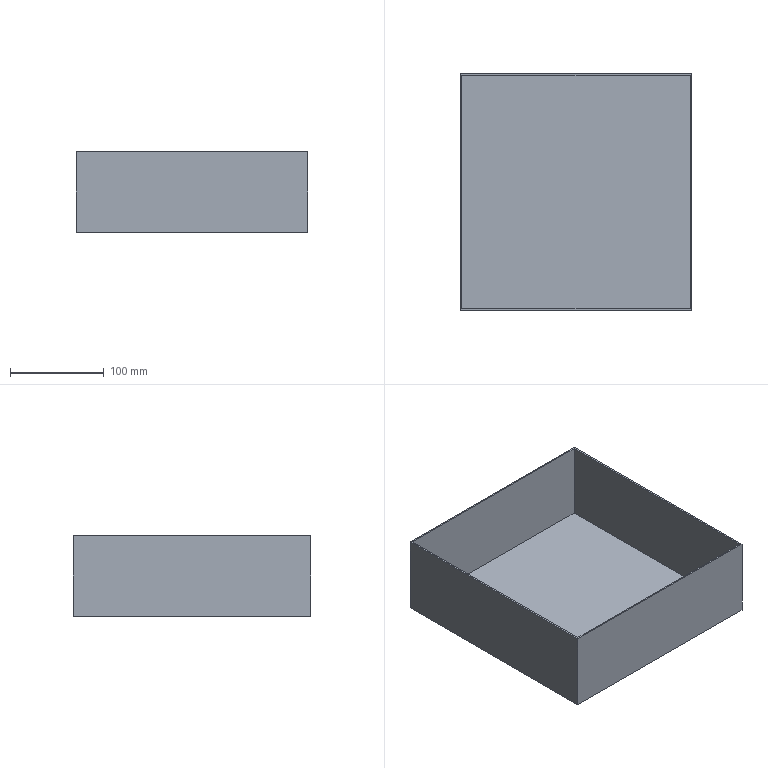Part | STEP file | 012-6-07-011 | 1 solid | 11 faces | box 247 x 253 x 86 mm | volume 291638 mm3 | plane 11
STEP:
#1=CARTESIAN_POINT('',(0.,0.,0.));
#2=DIRECTION('',(0.,0.,1.));
#3=DIRECTION('',(1.,0.,0.));
#4=AXIS2_PLACEMENT_3D('',#1,#2,#3);
#5=CARTESIAN_POINT('',(123.5,-126.5,0.));
#6=VERTEX_POINT('',#5);
#7=CARTESIAN_POINT('',(123.5,126.5,0.));
#8=VERTEX_POINT('',#7);
#9=CARTESIAN_POINT('',(123.5,126.5,0.));
#10=DIRECTION('',(0.,1.,0.));
#11=VECTOR('',#10,1.);
#12=LINE('',#9,#11);
#13=CARTESIAN_POINT('',(123.5,126.5,86.));
#14=DIRECTION('',(-1.,0.,0.));
#15=DIRECTION('',(0.,-1.,0.));
#16=AXIS2_PLACEMENT_3D('',#13,#14,#15);
#17=PLANE('',#16);
#18=CARTESIAN_POINT('',(0.,-86.));
#19=DIRECTION('',(-1.,0.));
#20=VECTOR('',#19,1.);
#21=LINE('',#18,#20);
#22=(GEOMETRIC_REPRESENTATION_CONTEXT(2)PARAMETRIC_REPRESENTATION_CONTEXT()REPRESENTATION_CONTEXT('',''));
#23=DEFINITIONAL_REPRESENTATION('',(#21),#22);
#24=PCURVE('',#17,#23);
#25=CARTESIAN_POINT('',(123.5,-126.5,0.));
#26=DIRECTION('',(0.,0.,1.));
#27=DIRECTION('',(1.,0.,0.));
#28=AXIS2_PLACEMENT_3D('',#25,#26,#27);
#29=PLANE('',#28);
#30=CARTESIAN_POINT('',(0.,253.));
#31=DIRECTION('',(0.,1.));
#32=VECTOR('',#31,1.);
#33=LINE('',#30,#32);
#34=(GEOMETRIC_REPRESENTATION_CONTEXT(2)PARAMETRIC_REPRESENTATION_CONTEXT()REPRESENTATION_CONTEXT('',''));
#35=DEFINITIONAL_REPRESENTATION('',(#33),#34);
#36=PCURVE('',#29,#35);
#37=SURFACE_CURVE('',#12,(#24,#36),.PCURVE_S1.);
#38=EDGE_CURVE('',#6,#8,#37,.T.);
#39=ORIENTED_EDGE('',*,*,#38,.T.);
#40=CARTESIAN_POINT('',(123.5,126.5,86.));
#41=VERTEX_POINT('',#40);
#42=CARTESIAN_POINT('',(123.5,126.5,86.));
#43=DIRECTION('',(0.,0.,-1.));
#44=VECTOR('',#43,1.);
#45=LINE('',#42,#44);
#46=CARTESIAN_POINT('',(0.,0.));
#47=DIRECTION('',(0.,-1.));
#48=VECTOR('',#47,1.);
#49=LINE('',#46,#48);
#50=(GEOMETRIC_REPRESENTATION_CONTEXT(2)PARAMETRIC_REPRESENTATION_CONTEXT()REPRESENTATION_CONTEXT('',''));
#51=DEFINITIONAL_REPRESENTATION('',(#49),#50);
#52=PCURVE('',#17,#51);
#53=CARTESIAN_POINT('',(-123.5,126.5,86.));
#54=DIRECTION('',(0.,-1.,0.));
#55=DIRECTION('',(0.,0.,-1.));
#56=AXIS2_PLACEMENT_3D('',#53,#54,#55);
#57=PLANE('',#56);
#58=CARTESIAN_POINT('',(0.,247.));
#59=DIRECTION('',(1.,0.));
#60=VECTOR('',#59,1.);
#61=LINE('',#58,#60);
#62=(GEOMETRIC_REPRESENTATION_CONTEXT(2)PARAMETRIC_REPRESENTATION_CONTEXT()REPRESENTATION_CONTEXT('',''));
#63=DEFINITIONAL_REPRESENTATION('',(#61),#62);
#64=PCURVE('',#57,#63);
#65=SURFACE_CURVE('',#45,(#52,#64),.PCURVE_S1.);
#66=EDGE_CURVE('',#41,#8,#65,.T.);
#67=ORIENTED_EDGE('',*,*,#66,.F.);
#68=CARTESIAN_POINT('',(123.5,-126.5,86.));
#69=VERTEX_POINT('',#68);
#70=CARTESIAN_POINT('',(123.5,126.5,86.));
#71=DIRECTION('',(0.,1.,0.));
#72=VECTOR('',#71,1.);
#73=LINE('',#70,#72);
#74=CARTESIAN_POINT('',(0.,0.));
#75=DIRECTION('',(-1.,0.));
#76=VECTOR('',#75,1.);
#77=LINE('',#74,#76);
#78=(GEOMETRIC_REPRESENTATION_CONTEXT(2)PARAMETRIC_REPRESENTATION_CONTEXT()REPRESENTATION_CONTEXT('',''));
#79=DEFINITIONAL_REPRESENTATION('',(#77),#78);
#80=PCURVE('',#17,#79);
#81=CARTESIAN_POINT('',(123.5,-126.5,86.));
#82=DIRECTION('',(0.,0.,1.));
#83=DIRECTION('',(1.,0.,0.));
#84=AXIS2_PLACEMENT_3D('',#81,#82,#83);
#85=PLANE('',#84);
#86=CARTESIAN_POINT('',(0.,253.));
#87=DIRECTION('',(0.,1.));
#88=VECTOR('',#87,1.);
#89=LINE('',#86,#88);
#90=(GEOMETRIC_REPRESENTATION_CONTEXT(2)PARAMETRIC_REPRESENTATION_CONTEXT()REPRESENTATION_CONTEXT('',''));
#91=DEFINITIONAL_REPRESENTATION('',(#89),#90);
#92=PCURVE('',#85,#91);
#93=SURFACE_CURVE('',#73,(#80,#92),.PCURVE_S1.);
#94=EDGE_CURVE('',#69,#41,#93,.T.);
#95=ORIENTED_EDGE('',*,*,#94,.F.);
#96=CARTESIAN_POINT('',(123.5,-126.5,86.));
#97=DIRECTION('',(0.,0.,-1.));
#98=VECTOR('',#97,1.);
#99=LINE('',#96,#98);
#100=CARTESIAN_POINT('',(253.,0.));
#101=DIRECTION('',(0.,-1.));
#102=VECTOR('',#101,1.);
#103=LINE('',#100,#102);
#104=(GEOMETRIC_REPRESENTATION_CONTEXT(2)PARAMETRIC_REPRESENTATION_CONTEXT()REPRESENTATION_CONTEXT('',''));
#105=DEFINITIONAL_REPRESENTATION('',(#103),#104);
#106=PCURVE('',#17,#105);
#107=CARTESIAN_POINT('',(-123.5,-126.5,86.));
#108=DIRECTION('',(0.,1.,0.));
#109=DIRECTION('',(0.,0.,1.));
#110=AXIS2_PLACEMENT_3D('',#107,#108,#109);
#111=PLANE('',#110);
#112=CARTESIAN_POINT('',(0.,247.));
#113=DIRECTION('',(-1.,0.));
#114=VECTOR('',#113,1.);
#115=LINE('',#112,#114);
#116=(GEOMETRIC_REPRESENTATION_CONTEXT(2)PARAMETRIC_REPRESENTATION_CONTEXT()REPRESENTATION_CONTEXT('',''));
#117=DEFINITIONAL_REPRESENTATION('',(#115),#116);
#118=PCURVE('',#111,#117);
#119=SURFACE_CURVE('',#99,(#106,#118),.PCURVE_S1.);
#120=EDGE_CURVE('',#69,#6,#119,.T.);
#121=ORIENTED_EDGE('',*,*,#120,.T.);
#122=EDGE_LOOP('',(#39,#67,#95,#121));
#123=FACE_BOUND('',#122,.T.);
#124=ADVANCED_FACE('',(#123),#17,.F.);
#125=CARTESIAN_POINT('',(-123.5,126.5,0.));
#126=VERTEX_POINT('',#125);
#127=CARTESIAN_POINT('',(-123.5,126.5,0.));
#128=DIRECTION('',(-1.,0.,0.));
#129=VECTOR('',#128,1.);
#130=LINE('',#127,#129);
#131=CARTESIAN_POINT('',(86.,0.));
#132=DIRECTION('',(0.,-1.));
#133=VECTOR('',#132,1.);
#134=LINE('',#131,#133);
#135=(GEOMETRIC_REPRESENTATION_CONTEXT(2)PARAMETRIC_REPRESENTATION_CONTEXT()REPRESENTATION_CONTEXT('',''));
#136=DEFINITIONAL_REPRESENTATION('',(#134),#135);
#137=PCURVE('',#57,#136);
#138=CARTESIAN_POINT('',(-247.,253.));
#139=DIRECTION('',(-1.,0.));
#140=VECTOR('',#139,1.);
#141=LINE('',#138,#140);
#142=(GEOMETRIC_REPRESENTATION_CONTEXT(2)PARAMETRIC_REPRESENTATION_CONTEXT()REPRESENTATION_CONTEXT('',''));
#143=DEFINITIONAL_REPRESENTATION('',(#141),#142);
#144=PCURVE('',#29,#143);
#145=SURFACE_CURVE('',#130,(#137,#144),.PCURVE_S1.);
#146=EDGE_CURVE('',#8,#126,#145,.T.);
#147=ORIENTED_EDGE('',*,*,#146,.T.);
#148=CARTESIAN_POINT('',(-123.5,126.5,86.));
#149=VERTEX_POINT('',#148);
#150=CARTESIAN_POINT('',(-123.5,126.5,86.));
#151=DIRECTION('',(0.,0.,-1.));
#152=VECTOR('',#151,1.);
#153=LINE('',#150,#152);
#154=CARTESIAN_POINT('',(0.,0.));
#155=DIRECTION('',(1.,0.));
#156=VECTOR('',#155,1.);
#157=LINE('',#154,#156);
#158=(GEOMETRIC_REPRESENTATION_CONTEXT(2)PARAMETRIC_REPRESENTATION_CONTEXT()REPRESENTATION_CONTEXT('',''));
#159=DEFINITIONAL_REPRESENTATION('',(#157),#158);
#160=PCURVE('',#57,#159);
#161=CARTESIAN_POINT('',(-123.5,126.5,86.));
#162=DIRECTION('',(1.,0.,0.));
#163=DIRECTION('',(0.,1.,0.));
#164=AXIS2_PLACEMENT_3D('',#161,#162,#163);
#165=PLANE('',#164);
#166=CARTESIAN_POINT('',(0.,0.));
#167=DIRECTION('',(0.,-1.));
#168=VECTOR('',#167,1.);
#169=LINE('',#166,#168);
#170=(GEOMETRIC_REPRESENTATION_CONTEXT(2)PARAMETRIC_REPRESENTATION_CONTEXT()REPRESENTATION_CONTEXT('',''));
#171=DEFINITIONAL_REPRESENTATION('',(#169),#170);
#172=PCURVE('',#165,#171);
#173=SURFACE_CURVE('',#153,(#160,#172),.PCURVE_S1.);
#174=EDGE_CURVE('',#149,#126,#173,.T.);
#175=ORIENTED_EDGE('',*,*,#174,.F.);
#176=CARTESIAN_POINT('',(-123.5,126.5,86.));
#177=DIRECTION('',(-1.,0.,0.));
#178=VECTOR('',#177,1.);
#179=LINE('',#176,#178);
#180=CARTESIAN_POINT('',(0.,0.));
#181=DIRECTION('',(0.,-1.));
#182=VECTOR('',#181,1.);
#183=LINE('',#180,#182);
#184=(GEOMETRIC_REPRESENTATION_CONTEXT(2)PARAMETRIC_REPRESENTATION_CONTEXT()REPRESENTATION_CONTEXT('',''));
#185=DEFINITIONAL_REPRESENTATION('',(#183),#184);
#186=PCURVE('',#57,#185);
#187=CARTESIAN_POINT('',(-247.,253.));
#188=DIRECTION('',(-1.,0.));
#189=VECTOR('',#188,1.);
#190=LINE('',#187,#189);
#191=(GEOMETRIC_REPRESENTATION_CONTEXT(2)PARAMETRIC_REPRESENTATION_CONTEXT()REPRESENTATION_CONTEXT('',''));
#192=DEFINITIONAL_REPRESENTATION('',(#190),#191);
#193=PCURVE('',#85,#192);
#194=SURFACE_CURVE('',#179,(#186,#193),.PCURVE_S1.);
#195=EDGE_CURVE('',#41,#149,#194,.T.);
#196=ORIENTED_EDGE('',*,*,#195,.F.);
#197=ORIENTED_EDGE('',*,*,#66,.T.);
#198=EDGE_LOOP('',(#147,#175,#196,#197));
#199=FACE_BOUND('',#198,.T.);
#200=ADVANCED_FACE('',(#199),#57,.F.);
#201=CARTESIAN_POINT('',(-123.5,-126.5,0.));
#202=VERTEX_POINT('',#201);
#203=CARTESIAN_POINT('',(-123.5,126.5,0.));
#204=DIRECTION('',(0.,-1.,0.));
#205=VECTOR('',#204,1.);
#206=LINE('',#203,#205);
#207=CARTESIAN_POINT('',(0.,-86.));
#208=DIRECTION('',(-1.,0.));
#209=VECTOR('',#208,1.);
#210=LINE('',#207,#209);
#211=(GEOMETRIC_REPRESENTATION_CONTEXT(2)PARAMETRIC_REPRESENTATION_CONTEXT()REPRESENTATION_CONTEXT('',''));
#212=DEFINITIONAL_REPRESENTATION('',(#210),#211);
#213=PCURVE('',#165,#212);
#214=CARTESIAN_POINT('',(-247.,253.));
#215=DIRECTION('',(0.,-1.));
#216=VECTOR('',#215,1.);
#217=LINE('',#214,#216);
#218=(GEOMETRIC_REPRESENTATION_CONTEXT(2)PARAMETRIC_REPRESENTATION_CONTEXT()REPRESENTATION_CONTEXT('',''));
#219=DEFINITIONAL_REPRESENTATION('',(#217),#218);
#220=PCURVE('',#29,#219);
#221=SURFACE_CURVE('',#206,(#213,#220),.PCURVE_S1.);
#222=EDGE_CURVE('',#126,#202,#221,.T.);
#223=ORIENTED_EDGE('',*,*,#222,.T.);
#224=CARTESIAN_POINT('',(-123.5,-126.5,86.));
#225=VERTEX_POINT('',#224);
#226=CARTESIAN_POINT('',(-123.5,-126.5,86.));
#227=DIRECTION('',(0.,0.,-1.));
#228=VECTOR('',#227,1.);
#229=LINE('',#226,#228);
#230=CARTESIAN_POINT('',(-253.,0.));
#231=DIRECTION('',(0.,-1.));
#232=VECTOR('',#231,1.);
#233=LINE('',#230,#232);
#234=(GEOMETRIC_REPRESENTATION_CONTEXT(2)PARAMETRIC_REPRESENTATION_CONTEXT()REPRESENTATION_CONTEXT('',''));
#235=DEFINITIONAL_REPRESENTATION('',(#233),#234);
#236=PCURVE('',#165,#235);
#237=CARTESIAN_POINT('',(0.,0.));
#238=DIRECTION('',(-1.,0.));
#239=VECTOR('',#238,1.);
#240=LINE('',#237,#239);
#241=(GEOMETRIC_REPRESENTATION_CONTEXT(2)PARAMETRIC_REPRESENTATION_CONTEXT()REPRESENTATION_CONTEXT('',''));
#242=DEFINITIONAL_REPRESENTATION('',(#240),#241);
#243=PCURVE('',#111,#242);
#244=SURFACE_CURVE('',#229,(#236,#243),.PCURVE_S1.);
#245=EDGE_CURVE('',#225,#202,#244,.T.);
#246=ORIENTED_EDGE('',*,*,#245,.F.);
#247=CARTESIAN_POINT('',(-123.5,126.5,86.));
#248=DIRECTION('',(0.,-1.,0.));
#249=VECTOR('',#248,1.);
#250=LINE('',#247,#249);
#251=CARTESIAN_POINT('',(0.,0.));
#252=DIRECTION('',(-1.,0.));
#253=VECTOR('',#252,1.);
#254=LINE('',#251,#253);
#255=(GEOMETRIC_REPRESENTATION_CONTEXT(2)PARAMETRIC_REPRESENTATION_CONTEXT()REPRESENTATION_CONTEXT('',''));
#256=DEFINITIONAL_REPRESENTATION('',(#254),#255);
#257=PCURVE('',#165,#256);
#258=CARTESIAN_POINT('',(-247.,253.));
#259=DIRECTION('',(0.,-1.));
#260=VECTOR('',#259,1.);
#261=LINE('',#258,#260);
#262=(GEOMETRIC_REPRESENTATION_CONTEXT(2)PARAMETRIC_REPRESENTATION_CONTEXT()REPRESENTATION_CONTEXT('',''));
#263=DEFINITIONAL_REPRESENTATION('',(#261),#262);
#264=PCURVE('',#85,#263);
#265=SURFACE_CURVE('',#250,(#257,#264),.PCURVE_S1.);
#266=EDGE_CURVE('',#149,#225,#265,.T.);
#267=ORIENTED_EDGE('',*,*,#266,.F.);
#268=ORIENTED_EDGE('',*,*,#174,.T.);
#269=EDGE_LOOP('',(#223,#246,#267,#268));
#270=FACE_BOUND('',#269,.T.);
#271=ADVANCED_FACE('',(#270),#165,.F.);
#272=CARTESIAN_POINT('',(-123.5,-126.5,0.));
#273=DIRECTION('',(1.,0.,0.));
#274=VECTOR('',#273,1.);
#275=LINE('',#272,#274);
#276=CARTESIAN_POINT('',(-86.,0.));
#277=DIRECTION('',(0.,1.));
#278=VECTOR('',#277,1.);
#279=LINE('',#276,#278);
#280=(GEOMETRIC_REPRESENTATION_CONTEXT(2)PARAMETRIC_REPRESENTATION_CONTEXT()REPRESENTATION_CONTEXT('',''));
#281=DEFINITIONAL_REPRESENTATION('',(#279),#280);
#282=PCURVE('',#111,#281);
#283=CARTESIAN_POINT('',(-247.,0.));
#284=DIRECTION('',(1.,0.));
#285=VECTOR('',#284,1.);
#286=LINE('',#283,#285);
#287=(GEOMETRIC_REPRESENTATION_CONTEXT(2)PARAMETRIC_REPRESENTATION_CONTEXT()REPRESENTATION_CONTEXT('',''));
#288=DEFINITIONAL_REPRESENTATION('',(#286),#287);
#289=PCURVE('',#29,#288);
#290=SURFACE_CURVE('',#275,(#282,#289),.PCURVE_S1.);
#291=EDGE_CURVE('',#202,#6,#290,.T.);
#292=ORIENTED_EDGE('',*,*,#291,.T.);
#293=ORIENTED_EDGE('',*,*,#120,.F.);
#294=CARTESIAN_POINT('',(-123.5,-126.5,86.));
#295=DIRECTION('',(1.,0.,0.));
#296=VECTOR('',#295,1.);
#297=LINE('',#294,#296);
#298=CARTESIAN_POINT('',(0.,0.));
#299=DIRECTION('',(0.,1.));
#300=VECTOR('',#299,1.);
#301=LINE('',#298,#300);
#302=(GEOMETRIC_REPRESENTATION_CONTEXT(2)PARAMETRIC_REPRESENTATION_CONTEXT()REPRESENTATION_CONTEXT('',''));
#303=DEFINITIONAL_REPRESENTATION('',(#301),#302);
#304=PCURVE('',#111,#303);
#305=CARTESIAN_POINT('',(-247.,0.));
#306=DIRECTION('',(1.,0.));
#307=VECTOR('',#306,1.);
#308=LINE('',#305,#307);
#309=(GEOMETRIC_REPRESENTATION_CONTEXT(2)PARAMETRIC_REPRESENTATION_CONTEXT()REPRESENTATION_CONTEXT('',''));
#310=DEFINITIONAL_REPRESENTATION('',(#308),#309);
#311=PCURVE('',#85,#310);
#312=SURFACE_CURVE('',#297,(#304,#311),.PCURVE_S1.);
#313=EDGE_CURVE('',#225,#69,#312,.T.);
#314=ORIENTED_EDGE('',*,*,#313,.F.);
#315=ORIENTED_EDGE('',*,*,#245,.T.);
#316=EDGE_LOOP('',(#292,#293,#314,#315));
#317=FACE_BOUND('',#316,.T.);
#318=ADVANCED_FACE('',(#317),#111,.F.);
#319=CARTESIAN_POINT('',(121.5,-124.5,86.));
#320=VERTEX_POINT('',#319);
#321=CARTESIAN_POINT('',(121.5,124.5,86.));
#322=VERTEX_POINT('',#321);
#323=CARTESIAN_POINT('',(121.5,126.5,86.));
#324=DIRECTION('',(0.,1.,0.));
#325=VECTOR('',#324,1.);
#326=LINE('',#323,#325);
#327=CARTESIAN_POINT('',(-2.,253.));
#328=DIRECTION('',(0.,1.));
#329=VECTOR('',#328,1.);
#330=LINE('',#327,#329);
#331=(GEOMETRIC_REPRESENTATION_CONTEXT(2)PARAMETRIC_REPRESENTATION_CONTEXT()REPRESENTATION_CONTEXT('',''));
#332=DEFINITIONAL_REPRESENTATION('',(#330),#331);
#333=PCURVE('',#85,#332);
#334=CARTESIAN_POINT('',(121.5,126.5,86.));
#335=DIRECTION('',(-1.,0.,0.));
#336=DIRECTION('',(0.,-1.,0.));
#337=AXIS2_PLACEMENT_3D('',#334,#335,#336);
#338=PLANE('',#337);
#339=CARTESIAN_POINT('',(0.,0.));
#340=DIRECTION('',(-1.,0.));
#341=VECTOR('',#340,1.);
#342=LINE('',#339,#341);
#343=(GEOMETRIC_REPRESENTATION_CONTEXT(2)PARAMETRIC_REPRESENTATION_CONTEXT()REPRESENTATION_CONTEXT('',''));
#344=DEFINITIONAL_REPRESENTATION('',(#342),#343);
#345=PCURVE('',#338,#344);
#346=SURFACE_CURVE('',#326,(#333,#345),.PCURVE_S1.);
#347=EDGE_CURVE('',#320,#322,#346,.T.);
#348=ORIENTED_EDGE('',*,*,#347,.F.);
#349=CARTESIAN_POINT('',(-121.5,-124.5,86.));
#350=VERTEX_POINT('',#349);
#351=CARTESIAN_POINT('',(-123.5,-124.5,86.));
#352=DIRECTION('',(1.,0.,0.));
#353=VECTOR('',#352,1.);
#354=LINE('',#351,#353);
#355=CARTESIAN_POINT('',(-247.,2.));
#356=DIRECTION('',(1.,0.));
#357=VECTOR('',#356,1.);
#358=LINE('',#355,#357);
#359=(GEOMETRIC_REPRESENTATION_CONTEXT(2)PARAMETRIC_REPRESENTATION_CONTEXT()REPRESENTATION_CONTEXT('',''));
#360=DEFINITIONAL_REPRESENTATION('',(#358),#359);
#361=PCURVE('',#85,#360);
#362=CARTESIAN_POINT('',(-123.5,-124.5,86.));
#363=DIRECTION('',(0.,1.,0.));
#364=DIRECTION('',(0.,0.,1.));
#365=AXIS2_PLACEMENT_3D('',#362,#363,#364);
#366=PLANE('',#365);
#367=CARTESIAN_POINT('',(0.,0.));
#368=DIRECTION('',(0.,1.));
#369=VECTOR('',#368,1.);
#370=LINE('',#367,#369);
#371=(GEOMETRIC_REPRESENTATION_CONTEXT(2)PARAMETRIC_REPRESENTATION_CONTEXT()REPRESENTATION_CONTEXT('',''));
#372=DEFINITIONAL_REPRESENTATION('',(#370),#371);
#373=PCURVE('',#366,#372);
#374=SURFACE_CURVE('',#354,(#361,#373),.PCURVE_S1.);
#375=EDGE_CURVE('',#350,#320,#374,.T.);
#376=ORIENTED_EDGE('',*,*,#375,.F.);
#377=CARTESIAN_POINT('',(-121.5,124.5,86.));
#378=VERTEX_POINT('',#377);
#379=CARTESIAN_POINT('',(-121.5,126.5,86.));
#380=DIRECTION('',(0.,-1.,0.));
#381=VECTOR('',#380,1.);
#382=LINE('',#379,#381);
#383=CARTESIAN_POINT('',(-245.,253.));
#384=DIRECTION('',(0.,-1.));
#385=VECTOR('',#384,1.);
#386=LINE('',#383,#385);
#387=(GEOMETRIC_REPRESENTATION_CONTEXT(2)PARAMETRIC_REPRESENTATION_CONTEXT()REPRESENTATION_CONTEXT('',''));
#388=DEFINITIONAL_REPRESENTATION('',(#386),#387);
#389=PCURVE('',#85,#388);
#390=CARTESIAN_POINT('',(-121.5,126.5,86.));
#391=DIRECTION('',(1.,0.,0.));
#392=DIRECTION('',(0.,1.,0.));
#393=AXIS2_PLACEMENT_3D('',#390,#391,#392);
#394=PLANE('',#393);
#395=CARTESIAN_POINT('',(0.,0.));
#396=DIRECTION('',(-1.,0.));
#397=VECTOR('',#396,1.);
#398=LINE('',#395,#397);
#399=(GEOMETRIC_REPRESENTATION_CONTEXT(2)PARAMETRIC_REPRESENTATION_CONTEXT()REPRESENTATION_CONTEXT('',''));
#400=DEFINITIONAL_REPRESENTATION('',(#398),#399);
#401=PCURVE('',#394,#400);
#402=SURFACE_CURVE('',#382,(#389,#401),.PCURVE_S1.);
#403=EDGE_CURVE('',#378,#350,#402,.T.);
#404=ORIENTED_EDGE('',*,*,#403,.F.);
#405=CARTESIAN_POINT('',(-123.5,124.5,86.));
#406=DIRECTION('',(-1.,0.,0.));
#407=VECTOR('',#406,1.);
#408=LINE('',#405,#407);
#409=CARTESIAN_POINT('',(-247.,251.));
#410=DIRECTION('',(-1.,0.));
#411=VECTOR('',#410,1.);
#412=LINE('',#409,#411);
#413=(GEOMETRIC_REPRESENTATION_CONTEXT(2)PARAMETRIC_REPRESENTATION_CONTEXT()REPRESENTATION_CONTEXT('',''));
#414=DEFINITIONAL_REPRESENTATION('',(#412),#413);
#415=PCURVE('',#85,#414);
#416=CARTESIAN_POINT('',(-123.5,124.5,86.));
#417=DIRECTION('',(0.,-1.,0.));
#418=DIRECTION('',(0.,0.,-1.));
#419=AXIS2_PLACEMENT_3D('',#416,#417,#418);
#420=PLANE('',#419);
#421=CARTESIAN_POINT('',(0.,0.));
#422=DIRECTION('',(0.,-1.));
#423=VECTOR('',#422,1.);
#424=LINE('',#421,#423);
#425=(GEOMETRIC_REPRESENTATION_CONTEXT(2)PARAMETRIC_REPRESENTATION_CONTEXT()REPRESENTATION_CONTEXT('',''));
#426=DEFINITIONAL_REPRESENTATION('',(#424),#425);
#427=PCURVE('',#420,#426);
#428=SURFACE_CURVE('',#408,(#415,#427),.PCURVE_S1.);
#429=EDGE_CURVE('',#322,#378,#428,.T.);
#430=ORIENTED_EDGE('',*,*,#429,.F.);
#431=EDGE_LOOP('',(#348,#376,#404,#430));
#432=FACE_BOUND('',#431,.T.);
#433=ORIENTED_EDGE('',*,*,#94,.T.);
#434=ORIENTED_EDGE('',*,*,#195,.T.);
#435=ORIENTED_EDGE('',*,*,#266,.T.);
#436=ORIENTED_EDGE('',*,*,#313,.T.);
#437=EDGE_LOOP('',(#433,#434,#435,#436));
#438=FACE_BOUND('',#437,.T.);
#439=ADVANCED_FACE('',(#432,#438),#85,.T.);
#440=ORIENTED_EDGE('',*,*,#38,.F.);
#441=ORIENTED_EDGE('',*,*,#291,.F.);
#442=ORIENTED_EDGE('',*,*,#222,.F.);
#443=ORIENTED_EDGE('',*,*,#146,.F.);
#444=EDGE_LOOP('',(#440,#441,#442,#443));
#445=FACE_BOUND('',#444,.T.);
#446=ADVANCED_FACE('',(#445),#29,.F.);
#447=CARTESIAN_POINT('',(121.5,-124.5,2.));
#448=VERTEX_POINT('',#447);
#449=CARTESIAN_POINT('',(121.5,124.5,2.));
#450=VERTEX_POINT('',#449);
#451=CARTESIAN_POINT('',(121.5,126.5,2.));
#452=DIRECTION('',(0.,1.,0.));
#453=VECTOR('',#452,1.);
#454=LINE('',#451,#453);
#455=CARTESIAN_POINT('',(0.,-84.));
#456=DIRECTION('',(-1.,0.));
#457=VECTOR('',#456,1.);
#458=LINE('',#455,#457);
#459=(GEOMETRIC_REPRESENTATION_CONTEXT(2)PARAMETRIC_REPRESENTATION_CONTEXT()REPRESENTATION_CONTEXT('',''));
#460=DEFINITIONAL_REPRESENTATION('',(#458),#459);
#461=PCURVE('',#338,#460);
#462=CARTESIAN_POINT('',(123.5,-126.5,2.));
#463=DIRECTION('',(0.,0.,1.));
#464=DIRECTION('',(1.,0.,0.));
#465=AXIS2_PLACEMENT_3D('',#462,#463,#464);
#466=PLANE('',#465);
#467=CARTESIAN_POINT('',(-2.,253.));
#468=DIRECTION('',(0.,1.));
#469=VECTOR('',#468,1.);
#470=LINE('',#467,#469);
#471=(GEOMETRIC_REPRESENTATION_CONTEXT(2)PARAMETRIC_REPRESENTATION_CONTEXT()REPRESENTATION_CONTEXT('',''));
#472=DEFINITIONAL_REPRESENTATION('',(#470),#471);
#473=PCURVE('',#466,#472);
#474=SURFACE_CURVE('',#454,(#461,#473),.PCURVE_S1.);
#475=EDGE_CURVE('',#448,#450,#474,.T.);
#476=ORIENTED_EDGE('',*,*,#475,.F.);
#477=CARTESIAN_POINT('',(121.5,-124.5,86.));
#478=DIRECTION('',(0.,0.,-1.));
#479=VECTOR('',#478,1.);
#480=LINE('',#477,#479);
#481=CARTESIAN_POINT('',(251.,0.));
#482=DIRECTION('',(0.,-1.));
#483=VECTOR('',#482,1.);
#484=LINE('',#481,#483);
#485=(GEOMETRIC_REPRESENTATION_CONTEXT(2)PARAMETRIC_REPRESENTATION_CONTEXT()REPRESENTATION_CONTEXT('',''));
#486=DEFINITIONAL_REPRESENTATION('',(#484),#485);
#487=PCURVE('',#338,#486);
#488=CARTESIAN_POINT('',(0.,245.));
#489=DIRECTION('',(-1.,0.));
#490=VECTOR('',#489,1.);
#491=LINE('',#488,#490);
#492=(GEOMETRIC_REPRESENTATION_CONTEXT(2)PARAMETRIC_REPRESENTATION_CONTEXT()REPRESENTATION_CONTEXT('',''));
#493=DEFINITIONAL_REPRESENTATION('',(#491),#492);
#494=PCURVE('',#366,#493);
#495=SURFACE_CURVE('',#480,(#487,#494),.PCURVE_S1.);
#496=EDGE_CURVE('',#320,#448,#495,.T.);
#497=ORIENTED_EDGE('',*,*,#496,.F.);
#498=ORIENTED_EDGE('',*,*,#347,.T.);
#499=CARTESIAN_POINT('',(121.5,124.5,86.));
#500=DIRECTION('',(0.,0.,-1.));
#501=VECTOR('',#500,1.);
#502=LINE('',#499,#501);
#503=CARTESIAN_POINT('',(2.,0.));
#504=DIRECTION('',(0.,-1.));
#505=VECTOR('',#504,1.);
#506=LINE('',#503,#505);
#507=(GEOMETRIC_REPRESENTATION_CONTEXT(2)PARAMETRIC_REPRESENTATION_CONTEXT()REPRESENTATION_CONTEXT('',''));
#508=DEFINITIONAL_REPRESENTATION('',(#506),#507);
#509=PCURVE('',#338,#508);
#510=CARTESIAN_POINT('',(0.,245.));
#511=DIRECTION('',(1.,0.));
#512=VECTOR('',#511,1.);
#513=LINE('',#510,#512);
#514=(GEOMETRIC_REPRESENTATION_CONTEXT(2)PARAMETRIC_REPRESENTATION_CONTEXT()REPRESENTATION_CONTEXT('',''));
#515=DEFINITIONAL_REPRESENTATION('',(#513),#514);
#516=PCURVE('',#420,#515);
#517=SURFACE_CURVE('',#502,(#509,#516),.PCURVE_S1.);
#518=EDGE_CURVE('',#322,#450,#517,.T.);
#519=ORIENTED_EDGE('',*,*,#518,.T.);
#520=EDGE_LOOP('',(#476,#497,#498,#519));
#521=FACE_BOUND('',#520,.T.);
#522=ADVANCED_FACE('',(#521),#338,.T.);
#523=CARTESIAN_POINT('',(-121.5,124.5,2.));
#524=VERTEX_POINT('',#523);
#525=CARTESIAN_POINT('',(-123.5,124.5,2.));
#526=DIRECTION('',(-1.,0.,0.));
#527=VECTOR('',#526,1.);
#528=LINE('',#525,#527);
#529=CARTESIAN_POINT('',(84.,0.));
#530=DIRECTION('',(0.,-1.));
#531=VECTOR('',#530,1.);
#532=LINE('',#529,#531);
#533=(GEOMETRIC_REPRESENTATION_CONTEXT(2)PARAMETRIC_REPRESENTATION_CONTEXT()REPRESENTATION_CONTEXT('',''));
#534=DEFINITIONAL_REPRESENTATION('',(#532),#533);
#535=PCURVE('',#420,#534);
#536=CARTESIAN_POINT('',(-247.,251.));
#537=DIRECTION('',(-1.,0.));
#538=VECTOR('',#537,1.);
#539=LINE('',#536,#538);
#540=(GEOMETRIC_REPRESENTATION_CONTEXT(2)PARAMETRIC_REPRESENTATION_CONTEXT()REPRESENTATION_CONTEXT('',''));
#541=DEFINITIONAL_REPRESENTATION('',(#539),#540);
#542=PCURVE('',#466,#541);
#543=SURFACE_CURVE('',#528,(#535,#542),.PCURVE_S1.);
#544=EDGE_CURVE('',#450,#524,#543,.T.);
#545=ORIENTED_EDGE('',*,*,#544,.F.);
#546=ORIENTED_EDGE('',*,*,#518,.F.);
#547=ORIENTED_EDGE('',*,*,#429,.T.);
#548=CARTESIAN_POINT('',(-121.5,124.5,86.));
#549=DIRECTION('',(0.,0.,-1.));
#550=VECTOR('',#549,1.);
#551=LINE('',#548,#550);
#552=CARTESIAN_POINT('',(0.,2.));
#553=DIRECTION('',(1.,0.));
#554=VECTOR('',#553,1.);
#555=LINE('',#552,#554);
#556=(GEOMETRIC_REPRESENTATION_CONTEXT(2)PARAMETRIC_REPRESENTATION_CONTEXT()REPRESENTATION_CONTEXT('',''));
#557=DEFINITIONAL_REPRESENTATION('',(#555),#556);
#558=PCURVE('',#420,#557);
#559=CARTESIAN_POINT('',(-2.,0.));
#560=DIRECTION('',(0.,-1.));
#561=VECTOR('',#560,1.);
#562=LINE('',#559,#561);
#563=(GEOMETRIC_REPRESENTATION_CONTEXT(2)PARAMETRIC_REPRESENTATION_CONTEXT()REPRESENTATION_CONTEXT('',''));
#564=DEFINITIONAL_REPRESENTATION('',(#562),#563);
#565=PCURVE('',#394,#564);
#566=SURFACE_CURVE('',#551,(#558,#565),.PCURVE_S1.);
#567=EDGE_CURVE('',#378,#524,#566,.T.);
#568=ORIENTED_EDGE('',*,*,#567,.T.);
#569=EDGE_LOOP('',(#545,#546,#547,#568));
#570=FACE_BOUND('',#569,.T.);
#571=ADVANCED_FACE('',(#570),#420,.T.);
#572=CARTESIAN_POINT('',(-121.5,-124.5,2.));
#573=VERTEX_POINT('',#572);
#574=CARTESIAN_POINT('',(-121.5,126.5,2.));
#575=DIRECTION('',(0.,-1.,0.));
#576=VECTOR('',#575,1.);
#577=LINE('',#574,#576);
#578=CARTESIAN_POINT('',(0.,-84.));
#579=DIRECTION('',(-1.,0.));
#580=VECTOR('',#579,1.);
#581=LINE('',#578,#580);
#582=(GEOMETRIC_REPRESENTATION_CONTEXT(2)PARAMETRIC_REPRESENTATION_CONTEXT()REPRESENTATION_CONTEXT('',''));
#583=DEFINITIONAL_REPRESENTATION('',(#581),#582);
#584=PCURVE('',#394,#583);
#585=CARTESIAN_POINT('',(-245.,253.));
#586=DIRECTION('',(0.,-1.));
#587=VECTOR('',#586,1.);
#588=LINE('',#585,#587);
#589=(GEOMETRIC_REPRESENTATION_CONTEXT(2)PARAMETRIC_REPRESENTATION_CONTEXT()REPRESENTATION_CONTEXT('',''));
#590=DEFINITIONAL_REPRESENTATION('',(#588),#589);
#591=PCURVE('',#466,#590);
#592=SURFACE_CURVE('',#577,(#584,#591),.PCURVE_S1.);
#593=EDGE_CURVE('',#524,#573,#592,.T.);
#594=ORIENTED_EDGE('',*,*,#593,.F.);
#595=ORIENTED_EDGE('',*,*,#567,.F.);
#596=ORIENTED_EDGE('',*,*,#403,.T.);
#597=CARTESIAN_POINT('',(-121.5,-124.5,86.));
#598=DIRECTION('',(0.,0.,-1.));
#599=VECTOR('',#598,1.);
#600=LINE('',#597,#599);
#601=CARTESIAN_POINT('',(-251.,0.));
#602=DIRECTION('',(0.,-1.));
#603=VECTOR('',#602,1.);
#604=LINE('',#601,#603);
#605=(GEOMETRIC_REPRESENTATION_CONTEXT(2)PARAMETRIC_REPRESENTATION_CONTEXT()REPRESENTATION_CONTEXT('',''));
#606=DEFINITIONAL_REPRESENTATION('',(#604),#605);
#607=PCURVE('',#394,#606);
#608=CARTESIAN_POINT('',(0.,2.));
#609=DIRECTION('',(-1.,0.));
#610=VECTOR('',#609,1.);
#611=LINE('',#608,#610);
#612=(GEOMETRIC_REPRESENTATION_CONTEXT(2)PARAMETRIC_REPRESENTATION_CONTEXT()REPRESENTATION_CONTEXT('',''));
#613=DEFINITIONAL_REPRESENTATION('',(#611),#612);
#614=PCURVE('',#366,#613);
#615=SURFACE_CURVE('',#600,(#607,#614),.PCURVE_S1.);
#616=EDGE_CURVE('',#350,#573,#615,.T.);
#617=ORIENTED_EDGE('',*,*,#616,.T.);
#618=EDGE_LOOP('',(#594,#595,#596,#617));
#619=FACE_BOUND('',#618,.T.);
#620=ADVANCED_FACE('',(#619),#394,.T.);
#621=CARTESIAN_POINT('',(-123.5,-124.5,2.));
#622=DIRECTION('',(1.,0.,0.));
#623=VECTOR('',#622,1.);
#624=LINE('',#621,#623);
#625=CARTESIAN_POINT('',(-84.,0.));
#626=DIRECTION('',(0.,1.));
#627=VECTOR('',#626,1.);
#628=LINE('',#625,#627);
#629=(GEOMETRIC_REPRESENTATION_CONTEXT(2)PARAMETRIC_REPRESENTATION_CONTEXT()REPRESENTATION_CONTEXT('',''));
#630=DEFINITIONAL_REPRESENTATION('',(#628),#629);
#631=PCURVE('',#366,#630);
#632=CARTESIAN_POINT('',(-247.,2.));
#633=DIRECTION('',(1.,0.));
#634=VECTOR('',#633,1.);
#635=LINE('',#632,#634);
#636=(GEOMETRIC_REPRESENTATION_CONTEXT(2)PARAMETRIC_REPRESENTATION_CONTEXT()REPRESENTATION_CONTEXT('',''));
#637=DEFINITIONAL_REPRESENTATION('',(#635),#636);
#638=PCURVE('',#466,#637);
#639=SURFACE_CURVE('',#624,(#631,#638),.PCURVE_S1.);
#640=EDGE_CURVE('',#573,#448,#639,.T.);
#641=ORIENTED_EDGE('',*,*,#640,.F.);
#642=ORIENTED_EDGE('',*,*,#616,.F.);
#643=ORIENTED_EDGE('',*,*,#375,.T.);
#644=ORIENTED_EDGE('',*,*,#496,.T.);
#645=EDGE_LOOP('',(#641,#642,#643,#644));
#646=FACE_BOUND('',#645,.T.);
#647=ADVANCED_FACE('',(#646),#366,.T.);
#648=ORIENTED_EDGE('',*,*,#475,.T.);
#649=ORIENTED_EDGE('',*,*,#544,.T.);
#650=ORIENTED_EDGE('',*,*,#593,.T.);
#651=ORIENTED_EDGE('',*,*,#640,.T.);
#652=EDGE_LOOP('',(#648,#649,#650,#651));
#653=FACE_BOUND('',#652,.T.);
#654=ADVANCED_FACE('',(#653),#466,.T.);
#655=CLOSED_SHELL('',(#124,#200,#271,#318,#439,#446,#522,#571,#620,#647,#654));
#656=MANIFOLD_SOLID_BREP('',#655);
#657=(LENGTH_UNIT()NAMED_UNIT(*)SI_UNIT(.MILLI.,.METRE.));
#658=UNCERTAINTY_MEASURE_WITH_UNIT(LENGTH_MEASURE(0.0000001),#657,'','');
#659=(NAMED_UNIT(*)PLANE_ANGLE_UNIT()SI_UNIT($,.RADIAN.));
#660=(NAMED_UNIT(*)SI_UNIT($,.STERADIAN.)SOLID_ANGLE_UNIT());
#661=(GEOMETRIC_REPRESENTATION_CONTEXT(3)GLOBAL_UNCERTAINTY_ASSIGNED_CONTEXT((#658))GLOBAL_UNIT_ASSIGNED_CONTEXT((#657,#659,#660))REPRESENTATION_CONTEXT('',''));
#662=ADVANCED_BREP_SHAPE_REPRESENTATION('',(#4,#656),#661);